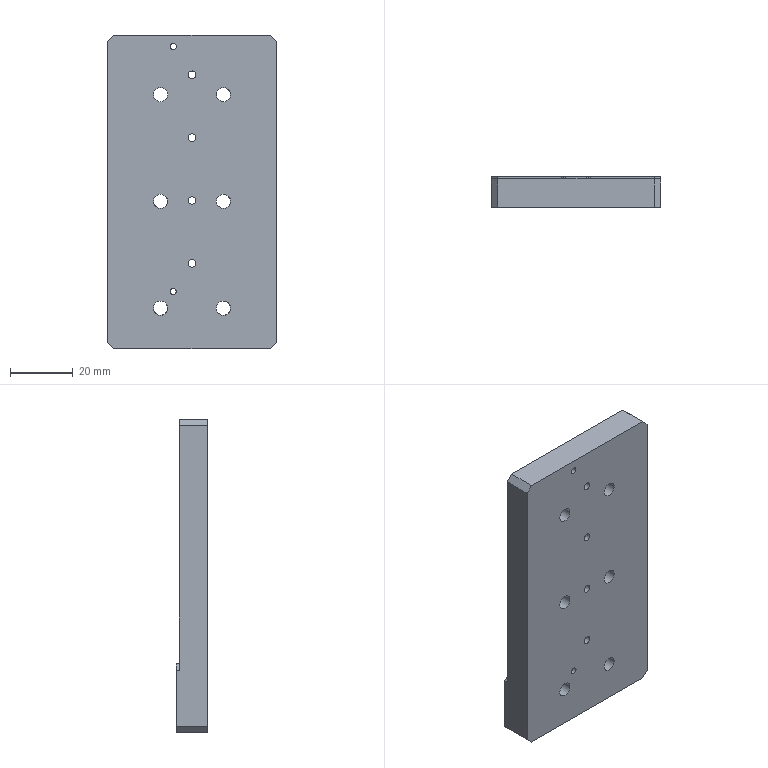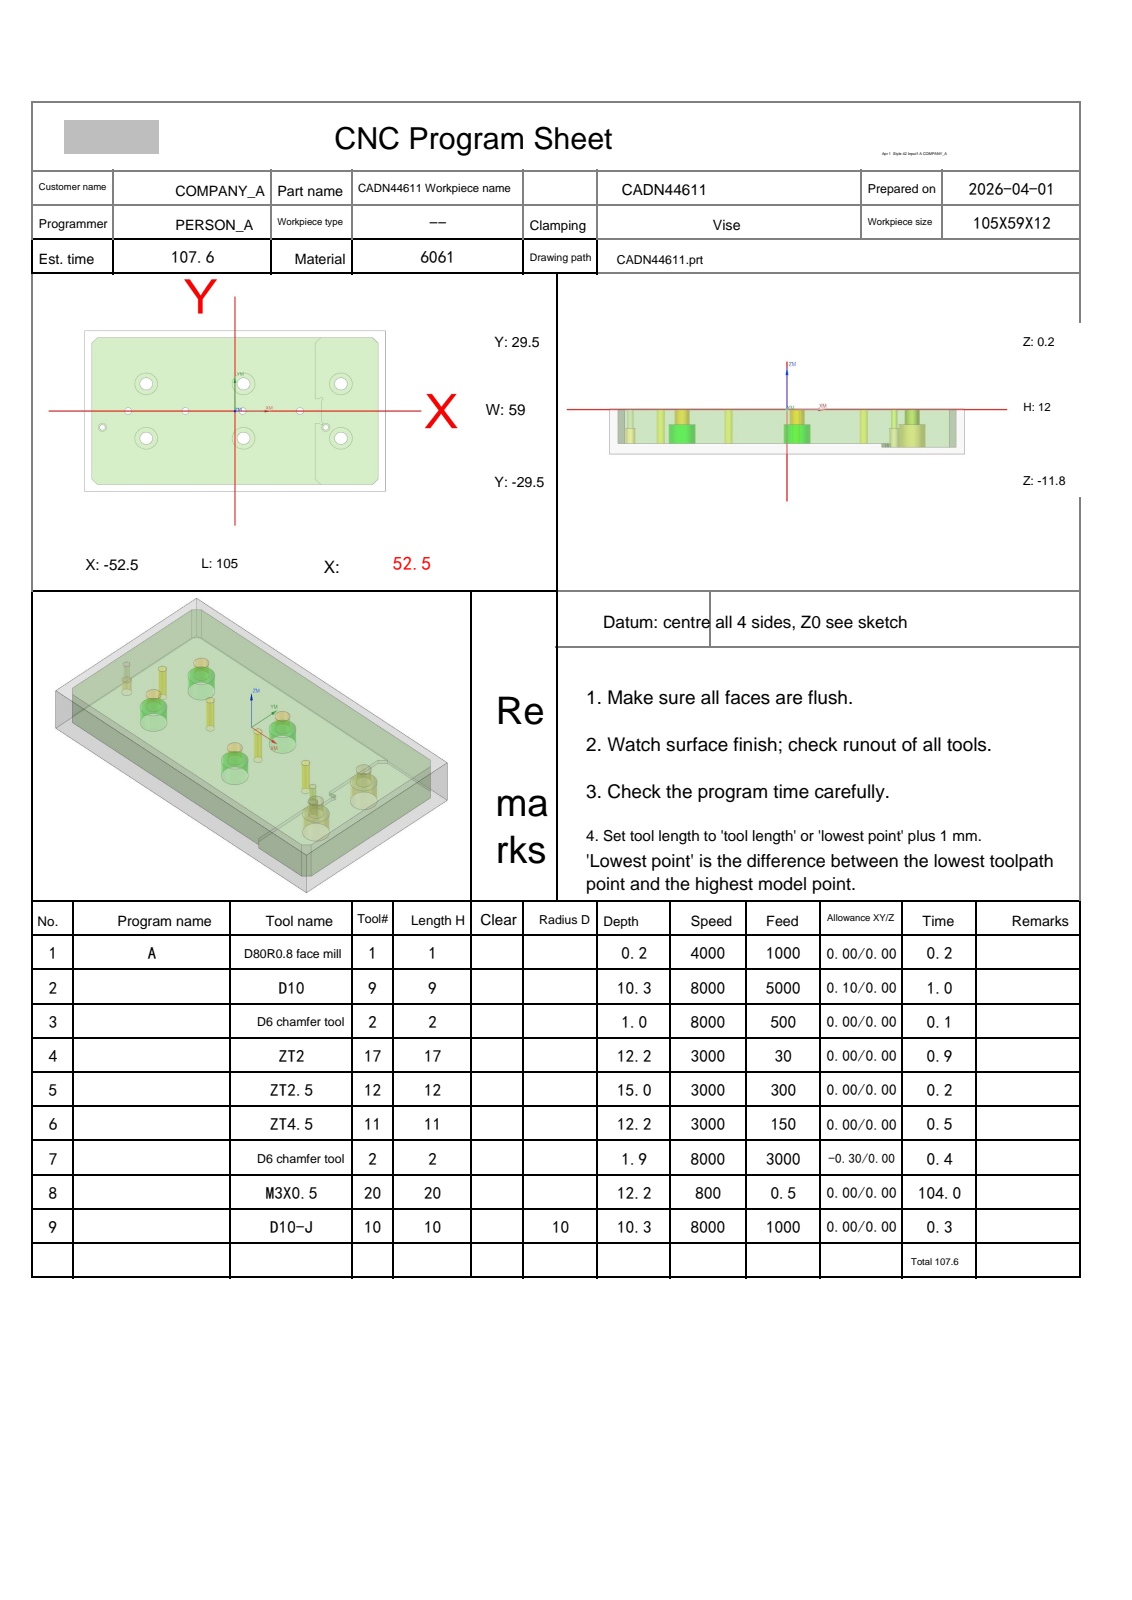NC program | NX | posted by the shop | part box 54 x 10 x 100 mm
Whole program:
%
O0001
(Machine time: 205.49 MIN)
(===Total Tool:8===)
(T1=D80R0.8 face mill D=80.  R=0.8  D-  H01 Z=-0.   )
(T9=D10     D=10.  R=0.   D-  H09 Z=-10.1 )
(T2=D6 chamfer tool   D=6.   R=0.   D-  H02 Z=-1.75 )
(T17=ZT2    D=2.   DR_a=118 D-  H17 Z=-12.  )
(T12=ZT2.5  D=2.5  DR_a=118 D-  H12 Z=-14.75)
(T11=ZT4.5  D=4.5  DR_a=118 D-  H11 Z=-12.  )
(T20=M3X0.5 D=2.5  DR_a=180 D-  H20 Z=-12.  )
(T10=D10-J  D=10.  R=0.   D10 H10 Z=-10.1 )
G80 G90 G17 G49 G40
G91 G28 Z0
M01
N1 T01 M06
(D80R0.8 face mill  D=80. R=0.8 H=01 ce=0.00 di=0.00)
G00 G90 G54 X95. Y0.0 M03 S4000
G43 H01 Z20.
M08
Z2.
G01 Z0.0 F1000.
X90.
X-90.
X-95.
Z2.
G00 Z20.
G91 G28 Z0.0
M05
M09
G91 G28 Z0.0
M01
N2 T09 M06
(D10  D=10. R=0. H=09 ce=0.10 di=0.00)
G00 G90 G54 X0.0 Y32.1 M03 S8000
G43 H09 Z20.
M08
Z.5
G01 X48. Z.392 F5000.
G02 X51.606 Y30.606 Z.383 I0.0 J-5.1
G01 X53.606 Y28.606 Z.376
G02 X55.1 Y25. Z.367 I-3.606 J-3.606
G01 Y-25. Z.254
G02 X53.606 Y-28.606 Z.245 I-5.1 J0.0
G01 X51.606 Y-30.606 Z.239
G02 X48. Y-32.1 Z.23 I-3.606 J3.606
G01 X-48. Z.013
G02 X-51.606 Y-30.606 Z.004 I0.0 J5.1
G01 X-53.606 Y-28.606 Z-.002
G02 X-55.1 Y-25. Z-.011 I3.606 J3.606
G01 Y25. Z-.124
G02 X-53.606 Y28.606 Z-.133 I5.1 J0.0
G01 X-51.606 Y30.606 Z-.14
G02 X-48. Y32.1 Z-.149 I3.606 J-3.606
G01 X48. Z-.366
G02 X51.606 Y30.606 Z-.375 I0.0 J-5.1
G01 X53.606 Y28.606 Z-.381
G02 X55.1 Y25. Z-.39 I-3.606 J-3.606
G01 Y-25. Z-.503
G02 X53.606 Y-28.606 Z-.512 I-5.1 J0.0
G01 X51.606 Y-30.606 Z-.518
G02 X48. Y-32.1 Z-.527 I-3.606 J3.606
G01 X-48. Z-.744
G02 X-51.606 Y-30.606 Z-.753 I0.0 J5.1
G01 X-53.606 Y-28.606 Z-.76
G02 X-55.1 Y-25. Z-.769 I3.606 J3.606
G01 Y25. Z-.881
G02 X-53.606 Y28.606 Z-.89 I5.1 J0.0
G01 X-51.606 Y30.606 Z-.897
G02 X-48. Y32.1 Z-.906 I3.606 J-3.606
G01 X48. Z-1.123
G02 X51.606 Y30.606 Z-1.132 I0.0 J-5.1
G01 X53.606 Y28.606 Z-1.138
G02 X55.1 Y25. Z-1.147 I-3.606 J-3.606
G01 Y-25. Z-1.26
G02 X53.606 Y-28.606 Z-1.269 I-5.1 J0.0
G01 X51.606 Y-30.606 Z-1.275
G02 X48. Y-32.1 Z-1.284 I-3.606 J3.606
G01 X-48. Z-1.501
G02 X-51.606 Y-30.606 Z-1.51 I0.0 J5.1
G01 X-53.606 Y-28.606 Z-1.517
G02 X-55.1 Y-25. Z-1.526 I3.606 J3.606
G01 Y25. Z-1.639
G02 X-53.606 Y28.606 Z-1.648 I5.1 J0.0
G01 X-51.606 Y30.606 Z-1.654
G02 X-48. Y32.1 Z-1.663 I3.606 J-3.606
G01 X48. Z-1.88
G02 X51.606 Y30.606 Z-1.889 I0.0 J-5.1
G01 X53.606 Y28.606 Z-1.895
G02 X55.1 Y25. Z-1.904 I-3.606 J-3.606
G01 Y-25. Z-2.017
G02 X53.606 Y-28.606 Z-2.026 I-5.1 J0.0
G01 X51.606 Y-30.606 Z-2.033
G02 X48. Y-32.1 Z-2.042 I-3.606 J3.606
G01 X-48. Z-2.258
G02 X-51.606 Y-30.606 Z-2.267 I0.0 J5.1
G01 X-53.606 Y-28.606 Z-2.274
G02 X-55.1 Y-25. Z-2.283 I3.606 J3.606
G01 Y25. Z-2.396
G02 X-53.606 Y28.606 Z-2.405 I5.1 J0.0
G01 X-51.606 Y30.606 Z-2.411
G02 X-48. Y32.1 Z-2.42 I3.606 J-3.606
G01 X48. Z-2.637
G02 X51.606 Y30.606 Z-2.646 I0.0 J-5.1
G01 X53.606 Y28.606 Z-2.652
G02 X55.1 Y25. Z-2.661 I-3.606 J-3.606
G01 Y-25. Z-2.774
G02 X53.606 Y-28.606 Z-2.783 I-5.1 J0.0
G01 X51.606 Y-30.606 Z-2.79
G02 X48. Y-32.1 Z-2.799 I-3.606 J3.606
G01 X-48. Z-3.016
G02 X-51.606 Y-30.606 Z-3.025 I0.0 J5.1
G01 X-53.606 Y-28.606 Z-3.031
G02 X-55.1 Y-25. Z-3.04 I3.606 J3.606
G01 Y25. Z-3.153
G02 X-53.606 Y28.606 Z-3.162 I5.1 J0.0
G01 X-51.606 Y30.606 Z-3.168
G02 X-48. Y32.1 Z-3.177 I3.606 J-3.606
G01 X48. Z-3.394
G02 X51.606 Y30.606 Z-3.403 I0.0 J-5.1
G01 X53.606 Y28.606 Z-3.41
G02 X55.1 Y25. Z-3.419 I-3.606 J-3.606
G01 Y-25. Z-3.531
G02 X53.606 Y-28.606 Z-3.54 I-5.1 J0.0
G01 X51.606 Y-30.606 Z-3.547
G02 X48. Y-32.1 Z-3.556 I-3.606 J3.606
G01 X-48. Z-3.773
G02 X-51.606 Y-30.606 Z-3.782 I0.0 J5.1
G01 X-53.606 Y-28.606 Z-3.788
G02 X-55.1 Y-25. Z-3.797 I3.606 J3.606
G01 Y25. Z-3.91
G02 X-53.606 Y28.606 Z-3.919 I5.1 J0.0
G01 X-51.606 Y30.606 Z-3.925
G02 X-48. Y32.1 Z-3.934 I3.606 J-3.606
G01 X48. Z-4.151
G02 X51.606 Y30.606 Z-4.16 I0.0 J-5.1
G01 X53.606 Y28.606 Z-4.167
G02 X55.1 Y25. Z-4.176 I-3.606 J-3.606
G01 Y-25. Z-4.289
G02 X53.606 Y-28.606 Z-4.298 I-5.1 J0.0
G01 X51.606 Y-30.606 Z-4.304
G02 X48. Y-32.1 Z-4.313 I-3.606 J3.606
G01 X-48. Z-4.53
G02 X-51.606 Y-30.606 Z-4.539 I0.0 J5.1
G01 X-53.606 Y-28.606 Z-4.545
G02 X-55.1 Y-25. Z-4.554 I3.606 J3.606
G01 Y25. Z-4.667
G02 X-53.606 Y28.606 Z-4.676 I5.1 J0.0
G01 X-51.606 Y30.606 Z-4.683
G02 X-48. Y32.1 Z-4.692 I3.606 J-3.606
G01 X48. Z-4.908
G02 X51.606 Y30.606 Z-4.917 I0.0 J-5.1
G01 X53.606 Y28.606 Z-4.924
G02 X55.1 Y25. Z-4.933 I-3.606 J-3.606
G01 Y-25. Z-5.046
G02 X53.606 Y-28.606 Z-5.055 I-5.1 J0.0
G01 X51.606 Y-30.606 Z-5.061
G02 X48. Y-32.1 Z-5.07 I-3.606 J3.606
G01 X-48. Z-5.287
G02 X-51.606 Y-30.606 Z-5.296 I0.0 J5.1
G01 X-53.606 Y-28.606 Z-5.302
G02 X-55.1 Y-25. Z-5.311 I3.606 J3.606
G01 Y25. Z-5.424
G02 X-53.606 Y28.606 Z-5.433 I5.1 J0.0
G01 X-51.606 Y30.606 Z-5.44
G02 X-48. Y32.1 Z-5.449 I3.606 J-3.606
G01 X48. Z-5.666
G02 X51.606 Y30.606 Z-5.675 I0.0 J-5.1
G01 X53.606 Y28.606 Z-5.681
G02 X55.1 Y25. Z-5.69 I-3.606 J-3.606
G01 Y-25. Z-5.803
G02 X53.606 Y-28.606 Z-5.812 I-5.1 J0.0
G01 X51.606 Y-30.606 Z-5.818
G02 X48. Y-32.1 Z-5.827 I-3.606 J3.606
G01 X-48. Z-6.044
G02 X-51.606 Y-30.606 Z-6.053 I0.0 J5.1
G01 X-53.606 Y-28.606 Z-6.06
G02 X-55.1 Y-25. Z-6.069 I3.606 J3.606
G01 Y25. Z-6.181
G02 X-53.606 Y28.606 Z-6.19 I5.1 J0.0
G01 X-51.606 Y30.606 Z-6.197
G02 X-48. Y32.1 Z-6.206 I3.606 J-3.606
G01 X48. Z-6.423
G02 X51.606 Y30.606 Z-6.432 I0.0 J-5.1
G01 X53.606 Y28.606 Z-6.438
G02 X55.1 Y25. Z-6.447 I-3.606 J-3.606
G01 Y-25. Z-6.56
G02 X53.606 Y-28.606 Z-6.569 I-5.1 J0.0
G01 X51.606 Y-30.606 Z-6.575
G02 X48. Y-32.1 Z-6.584 I-3.606 J3.606
G01 X-48. Z-6.801
G02 X-51.606 Y-30.606 Z-6.81 I0.0 J5.1
G01 X-53.606 Y-28.606 Z-6.817
G02 X-55.1 Y-25. Z-6.826 I3.606 J3.606
G01 Y25. Z-6.939
G02 X-53.606 Y28.606 Z-6.948 I5.1 J0.0
G01 X-51.606 Y30.606 Z-6.954
G02 X-48. Y32.1 Z-6.963 I3.606 J-3.606
G01 X48. Z-7.18
G02 X51.606 Y30.606 Z-7.189 I0.0 J-5.1
G01 X53.606 Y28.606 Z-7.195
G02 X55.1 Y25. Z-7.204 I-3.606 J-3.606
G01 Y-25. Z-7.317
G02 X53.606 Y-28.606 Z-7.326 I-5.1 J0.0
G01 X51.606 Y-30.606 Z-7.333
G02 X48. Y-32.1 Z-7.342 I-3.606 J3.606
G01 X-48. Z-7.558
G02 X-51.606 Y-30.606 Z-7.567 I0.0 J5.1
G01 X-53.606 Y-28.606 Z-7.574
G02 X-55.1 Y-25. Z-7.583 I3.606 J3.606
G01 Y25. Z-7.696
G02 X-53.606 Y28.606 Z-7.705 I5.1 J0.0
G01 X-51.606 Y30.606 Z-7.711
G02 X-48. Y32.1 Z-7.72 I3.606 J-3.606
G01 X48. Z-7.937
G02 X51.606 Y30.606 Z-7.946 I0.0 J-5.1
G01 X53.606 Y28.606 Z-7.952
G02 X55.1 Y25. Z-7.961 I-3.606 J-3.606
G01 Y-25. Z-8.074
G02 X53.606 Y-28.606 Z-8.083 I-5.1 J0.0
G01 X51.606 Y-30.606 Z-8.09
G02 X48. Y-32.1 Z-8.099 I-3.606 J3.606
G01 X-48. Z-8.316
G02 X-51.606 Y-30.606 Z-8.325 I0.0 J5.1
G01 X-53.606 Y-28.606 Z-8.331
G02 X-55.1 Y-25. Z-8.34 I3.606 J3.606
G01 Y25. Z-8.453
G02 X-53.606 Y28.606 Z-8.462 I5.1 J0.0
G01 X-51.606 Y30.606 Z-8.468
G02 X-48. Y32.1 Z-8.477 I3.606 J-3.606
G01 X48. Z-8.694
G02 X51.606 Y30.606 Z-8.703 I0.0 J-5.1
G01 X53.606 Y28.606 Z-8.71
G02 X55.1 Y25. Z-8.719 I-3.606 J-3.606
G01 Y-25. Z-8.831
G02 X53.606 Y-28.606 Z-8.84 I-5.1 J0.0
G01 X51.606 Y-30.606 Z-8.847
G02 X48. Y-32.1 Z-8.856 I-3.606 J3.606
G01 X-48. Z-9.073
G02 X-51.606 Y-30.606 Z-9.082 I0.0 J5.1
G01 X-53.606 Y-28.606 Z-9.088
G02 X-55.1 Y-25. Z-9.097 I3.606 J3.606
G01 Y25. Z-9.21
G02 X-53.606 Y28.606 Z-9.219 I5.1 J0.0
G01 X-51.606 Y30.606 Z-9.225
G02 X-48. Y32.1 Z-9.234 I3.606 J-3.606
G01 X48. Z-9.451
G02 X51.606 Y30.606 Z-9.46 I0.0 J-5.1
G01 X53.606 Y28.606 Z-9.467
G02 X55.1 Y25. Z-9.476 I-3.606 J-3.606
G01 Y-25. Z-9.589
G02 X53.606 Y-28.606 Z-9.598 I-5.1 J0.0
G01 X51.606 Y-30.606 Z-9.604
G02 X48. Y-32.1 Z-9.613 I-3.606 J3.606
G01 X-48. Z-9.83
G02 X-51.606 Y-30.606 Z-9.839 I0.0 J5.1
G01 X-53.606 Y-28.606 Z-9.845
G02 X-55.1 Y-25. Z-9.854 I3.606 J3.606
G01 Y25. Z-9.967
G02 X-53.606 Y28.606 Z-9.976 I5.1 J0.0
G01 X-51.606 Y30.606 Z-9.983
G02 X-48. Y32.1 Z-9.992 I3.606 J-3.606
G01 X0.0 Z-10.1
X48.
G02 X51.606 Y30.606 I0.0 J-5.1
G01 X53.606 Y28.606
G02 X55.1 Y25. I-3.606 J-3.606
G01 Y-25.
G02 X53.606 Y-28.606 I-5.1 J0.0
G01 X51.606 Y-30.606
G02 X48. Y-32.1 I-3.606 J3.606
G01 X-48.
G02 X-51.606 Y-30.606 I0.0 J5.1
G01 X-53.606 Y-28.606
G02 X-55.1 Y-25. I3.606 J3.606
G01 Y25.
G02 X-53.606 Y28.606 I5.1 J0.0
G01 X-51.606 Y30.606
G02 X-48. Y32.1 I3.606 J-3.606
G01 X0.0
X.5
Z-9.1
G00 Z20.
G91 G28 Z0.0
M05
M09
G91 G28 Z0.0
M01
N3 T02 M06
(D6 chamfer tool  D=6. R=0. H=02 ce=0.00 di=0.00)
G00 G90 G54 X37. Y10. M03 S8000
G43 H02 Z20.
M08
G98 G81 X37. Y10. Z-.8 R1. F500.
Y-10.
X31.701 Y-6.
X22.701 Y0.0
X3. Y10.
X2.701 Y0.0
X3. Y-10.
X-17.299 Y0.0
X-31. Y10.
X-37.299 Y0.0
X-46.299 Y-6.
X-31. Y-10.
G80
G00 Z20.
G91 G28 Z0.0
M05
M09
G91 G28 Z0.0
M01
N4 T17 M06
(ZT2 D=2. DR_a=118 H=17)
G00 G90 G54 X-46.299 Y-6. M03 S3000
G43 H17 Z20.
M08
G98 G83 X-46.299 Y-6. Z-12. R1. F30. Q1.5
X31.701
G80
G00 Z20.
G91 G28 Z0.0
M05
M09
G91 G28 Z0.0
M01
N5 T12 M06
(ZT2.5 D=2.5 DR_a=118 H=12)
G00 G90 G54 X-37.299 Y0.0 M03 S3000
G43 H12 Z20.
M08
G98 G83 X-37.299 Y0.0 Z-14.751 R1. F300. Q2.
X-17.299
X2.701
X22.701
G80
G00 Z20.
G91 G28 Z0.0
M05
M09
G91 G28 Z0.0
M01
N6 T11 M06
(ZT4.5 D=4.5 DR_a=118 H=11)
G00 G90 G54 X-31. Y10. M03 S3000
G43 H11 Z20.
M08
G98 G83 X-31. Y10. Z-12. R1. F150. Q3.
Y-10.
X3.
Y10.
X37.
Y-10.
G80
G00 Z20.
G91 G28 Z0.0
M05
M09
G91 G28 Z0.0
M01
N7 T02 M06
(D6 chamfer tool  D=6. R=0. H=02 ce=0.00 di=0.00)
G00 G90 G54 X-.25 Y29.128 M03 S8000
G43 H02 Z20.
M08
Z2.099
G01 Z-1.499 F3000.
G03 X-.33 Y28.828 I.52 J-.3
X-.03 Y28.308 I.6 J0.0
G01 X0.0 Y28.3
X48.
X48.254 Y28.275
X48.497 Y28.201
X48.722 Y28.081
X48.919 Y27.919
X50.919 Y25.919
X51.081 Y25.722
X51.201 Y25.497
X51.275 Y25.254
X51.3 Y25.
Y-25.
X51.275 Y-25.254
X51.201 Y-25.497
X51.081 Y-25.722
X50.919 Y-25.919
X48.919 Y-27.919
X48.722 Y-28.081
X48.497 Y-28.201
X48.254 Y-28.275
X48. Y-28.3
X-48.
X-48.254 Y-28.275
X-48.497 Y-28.201
X-48.722 Y-28.081
X-48.919 Y-27.919
X-50.919 Y-25.919
X-51.081 Y-25.722
X-51.201 Y-25.497
X-51.275 Y-25.254
X-51.3 Y-25.
Y25.
X-51.275 Y25.254
X-51.201 Y25.497
X-51.081 Y25.722
X-50.919 Y25.919
X-48.919 Y27.919
X-48.722 Y28.081
X-48.497 Y28.201
X-48.254 Y28.275
X-48. Y28.3
X0.0
X.03 Y28.308
G03 X.33 Y28.828 I-.3 J.52
X.25 Y29.128 I-.6 J0.0
G01 Z2.099
G00 Z20.
G00 G90 X-46.299 Y-6. M03 S8000
Z20.
G98 G81 X-46.299 Y-6. Z-1.3 R3. F500.
X31.701
G80
G00 Z20.
G00 G90 X-37.299 Y0.0 M03 S8000
Z20.
G98 G81 X-37.299 Y0.0 Z-1.75 R3. F500.
X-17.299
X2.701
X22.701
G80
G00 Z20.
G00 G90 X36.982 Y-9.45 M03 S8000
Z20.
Z-.5
G01 Z-1. F500.
X36.95 Y-8.5
G03 X35.45 Y-10. I0.0 J-1.5
X37. Y-11.55 I1.55 J0.0
X38.55 Y-10. I0.0 J1.55
X37. Y-8.45 I-1.55 J0.0
X35.45 Y-10. I0.0 J-1.55
X36.95 Y-11.5 I1.5 J0.0
G01 X36.982 Y-10.55
Z-.5
G00 Z20.
Y10.55
Z-.5
G01 Z-1.
X36.95 Y11.5
G03 X35.45 Y10. I0.0 J-1.5
X37. Y8.45 I1.55 J0.0
X38.55 Y10. I0.0 J1.55
X37. Y11.55 I-1.55 J0.0
X35.45 Y10. I0.0 J-1.55
X36.95 Y8.5 I1.5 J0.0
G01 X36.982 Y9.45
Z-.5
G00 Z20.
X2.982 Y10.55
Z-.5
G01 Z-1.
X2.95 Y11.5
G03 X1.45 Y10. I0.0 J-1.5
X3. Y8.45 I1.55 J0.0
X4.55 Y10. I0.0 J1.55
X3. Y11.55 I-1.55 J0.0
X1.45 Y10. I0.0 J-1.55
X2.95 Y8.5 I1.5 J0.0
G01 X2.982 Y9.45
Z-.5
G00 Z20.
Y-9.45
Z-.5
G01 Z-1.
X2.95 Y-8.5
G03 X1.45 Y-10. I0.0 J-1.5
X3. Y-11.55 I1.55 J0.0
X4.55 Y-10. I0.0 J1.55
X3. Y-8.45 I-1.55 J0.0
X1.45 Y-10. I0.0 J-1.55
X2.95 Y-11.5 I1.5 J0.0
G01 X2.982 Y-10.55
Z-.5
G00 Z20.
X-31.018 Y-9.45
Z-.5
G01 Z-1.
X-31.05 Y-8.5
G03 X-32.55 Y-10. I0.0 J-1.5
X-31. Y-11.55 I1.55 J0.0
X-29.45 Y-10. I0.0 J1.55
X-31. Y-8.45 I-1.55 J0.0
X-32.55 Y-10. I0.0 J-1.55
X-31.05 Y-11.5 I1.5 J0.0
G01 X-31.018 Y-10.55
Z-.5
G00 Z20.
Y10.55
Z-.5
G01 Z-1.
X-31.05 Y11.5
G03 X-32.55 Y10. I0.0 J-1.5
X-31. Y8.45 I1.55 J0.0
X-29.45 Y10. I0.0 J1.55
X-31. Y11.55 I-1.55 J0.0
X-32.55 Y10. I0.0 J-1.55
X-31.05 Y8.5 I1.5 J0.0
G01 X-31.018 Y9.45
Z-.5
G00 Z20.
G91 G28 Z0.0
M05
M09
G91 G28 Z0.0
M01
N8 T20 M06
(M3X0.5 D=2.5 DR_a=180 H=20)
G00 G90 G54 X-37.299 Y0.0 M03 S800
G43 H20 Z20.
M08
G95
G98 G84 X-37.299 Y0.0 Z-12. R1. F.5 Q5.
X-17.299
X2.701
X22.701
G80
G94
G00 Z20.
G91 G28 Z0.0
M05
M09
G91 G28 Z0.0
M01
N9 T10 M06
(D10-J  D=10. R=0. H=10 ce=0.00 di=0.00)
G00 G90 G54 X-49.013 Y33.116 M03 S8000
G43 H10 Z20.
M08
Z-9.6
G01 Z-10.1 F1000.
G41 D10
X-48.997 Y32.917
G03 X-48. Y32. I.997 J.083
G01 X48.
G02 X51.536 Y30.536 I0.0 J-5.
G01 X53.536 Y28.536
G02 X55. Y25. I-3.536 J-3.536
G01 Y-25.
G02 X53.536 Y-28.536 I-5. J0.0
G01 X51.536 Y-30.536
G02 X48. Y-32. I-3.536 J3.536
G01 X-48.
G02 X-51.536 Y-30.536 I0.0 J5.
G01 X-53.536 Y-28.536
G02 X-55. Y-25. I3.536 J3.536
G01 Y25.
G02 X-53.536 Y28.536 I5. J0.0
G01 X-51.536 Y30.536
G02 X-48. Y32. I3.536 J-3.536
G01 X-47.5
G03 X-46.5 Y33. I0.0 J1.
G01 G40 Y33.2
Z-9.6
G00 Z20.
M05
M09
G91 G28 Z0.0
G91 G28 Y0.0
M30
%